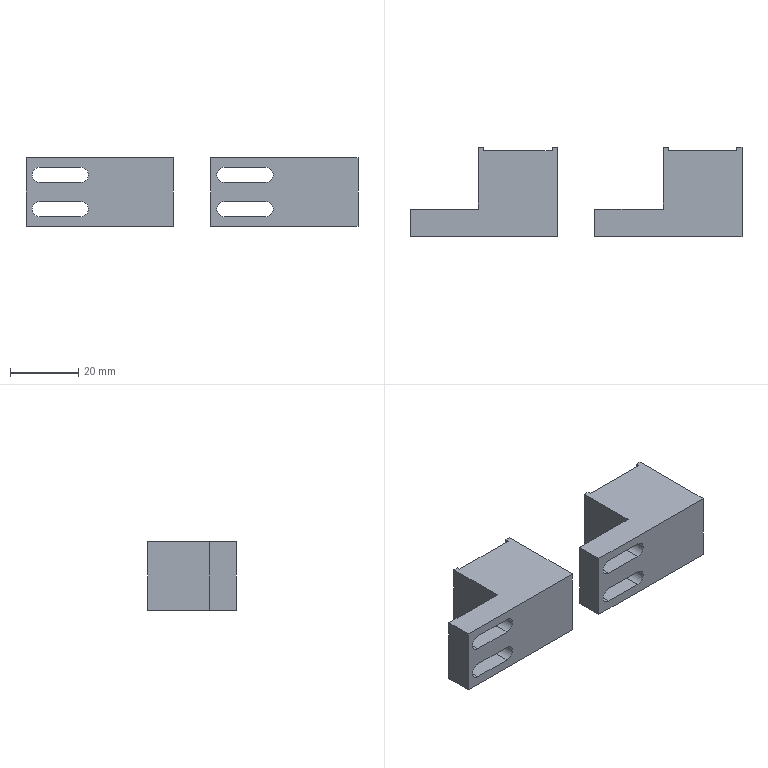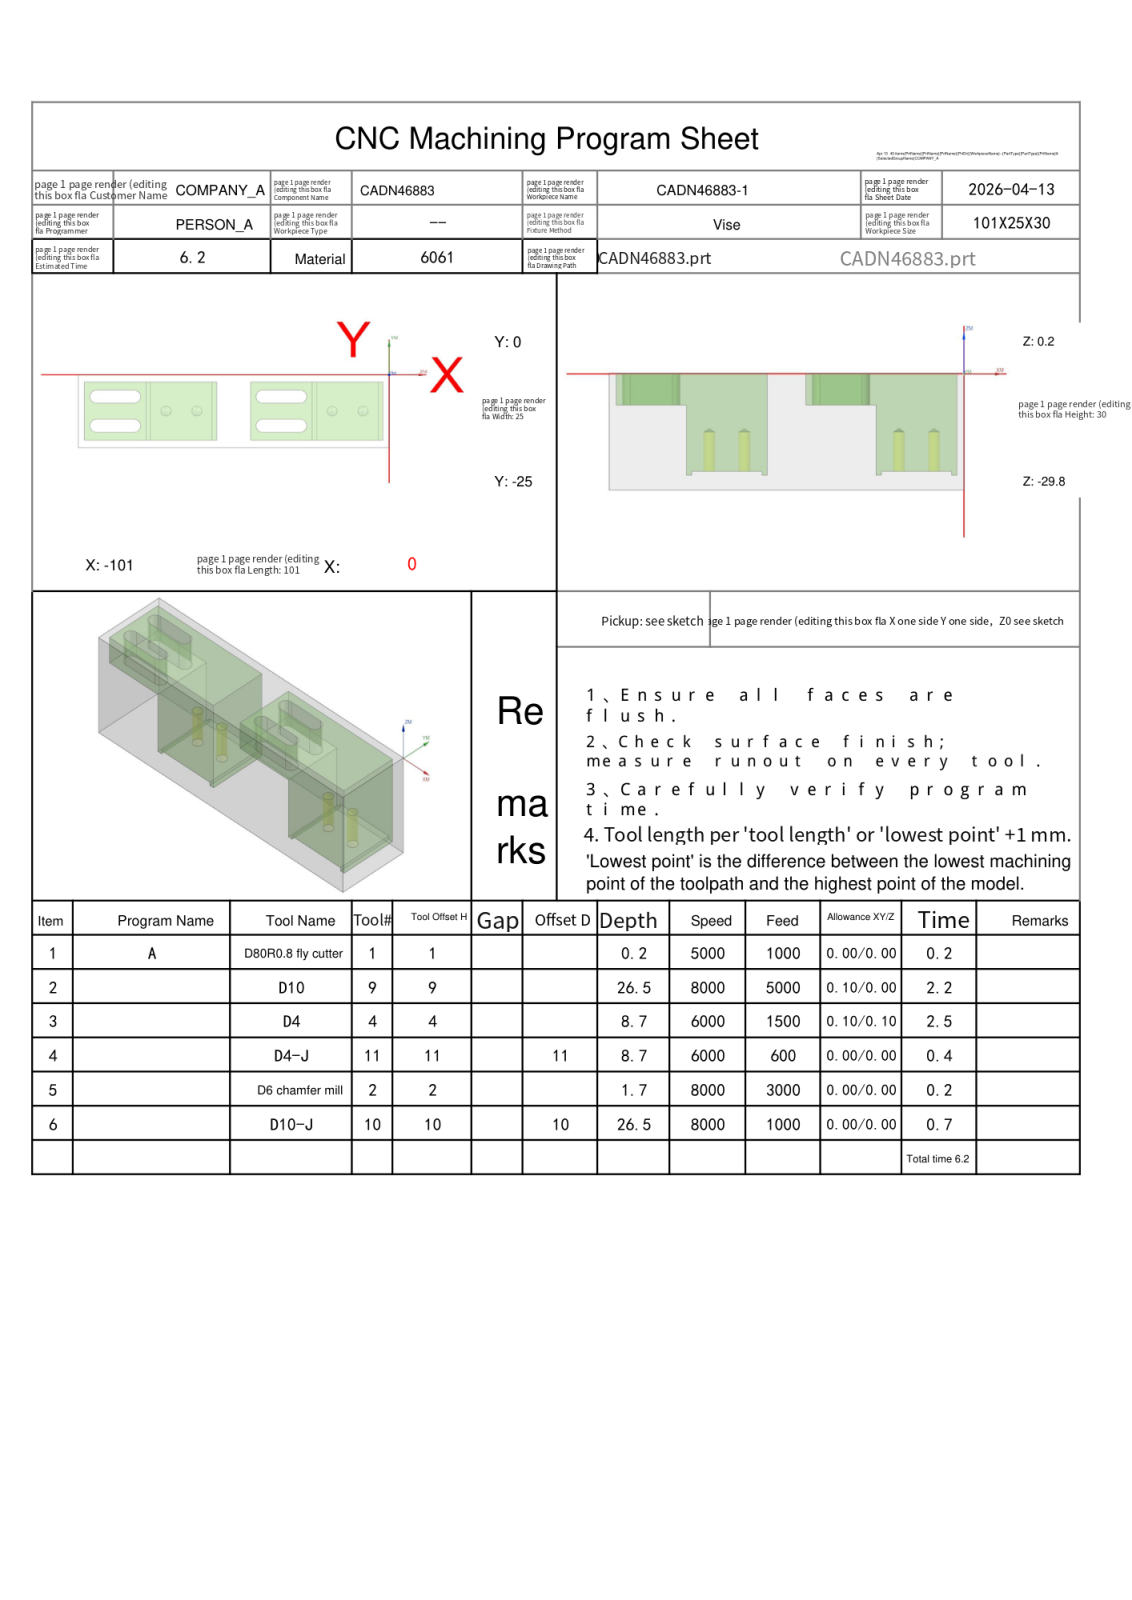NC program | NX | posted by the shop | part box 97 x 26 x 20 mm
Lines 1 to 1841 of 2082, first 1269 of 1839 lines:
%
O0001
(Machine time: 7.36 MIN)
(===Total Tool:6===)
(T1=D80R0.8 fly cutter D=80.  R=0.8  D-  H01 Z=0.    )
(T9=D10     D=10.  R=0.   D-  H09 Z=-26.3 )
(T4=D4      D=4.   R=0.   D-  H04 Z=-8.5  )
(T11=D4-J   D=4.   R=0.   D11 H11 Z=-8.5  )
(T2=D6 chamfer mill   D=6.   R=0.   D-  H02 Z=-1.5  )
(T10=D10-J  D=10.  R=0.   D10 H10 Z=-26.3 )
G80 G90 G17 G49 G40
G91 G28 Z0
M01
N1 T01 M06
(D80R0.8 fly cutter  D=80. R=0.8 H=01 ce=0.00 di=0.00)
(MAX_Z=20. MIN_Z=0. Time=0.20M)
G00 G90 G54 X43. Y-12.5 M03 S5000
G43 H01 Z20.
M08
Z2.
G01 Z0.0 F1000.
X38.
X-139.
X-144.
Z2.
G00 Z20.
G91 G28 Z0.0
M05
M09
G91 G28 Z0.0
M01
N2 T09 M06
(D10  D=10. R=0. H=09 ce=0.10 di=0.00)
(MAX_Z=20. MIN_Z=-26.3 Time=2.23M)
G00 G90 G54 X-77.5 Y-27.6 M03 S8000
G43 H09 Z20.
M08
Z.5
G01 X-99. Z.393 F5000.
G02 X-104.1 Y-22.5 Z.353 I0.0 J5.1
G01 Y-2.5 Z.253
G02 X-99. Y2.6 Z.213 I5.1 J0.0
G01 X-56. Z-.001
G02 X-50.9 Y-2.5 Z-.041 I0.0 J-5.1
G01 Y-22.5 Z-.141
G02 X-56. Y-27.6 Z-.181 I-5.1 J0.0
G01 X-99. Z-.395
G02 X-104.1 Y-22.5 Z-.435 I0.0 J5.1
G01 Y-2.5 Z-.535
G02 X-99. Y2.6 Z-.575 I5.1 J0.0
G01 X-56. Z-.79
G02 X-50.9 Y-2.5 Z-.83 I0.0 J-5.1
G01 Y-22.5 Z-.929
G02 X-56. Y-27.6 Z-.969 I-5.1 J0.0
G01 X-99. Z-1.184
G02 X-104.1 Y-22.5 Z-1.224 I0.0 J5.1
G01 Y-2.5 Z-1.323
G02 X-99. Y2.6 Z-1.363 I5.1 J0.0
G01 X-56. Z-1.578
G02 X-50.9 Y-2.5 Z-1.618 I0.0 J-5.1
G01 Y-22.5 Z-1.718
G02 X-56. Y-27.6 Z-1.757 I-5.1 J0.0
G01 X-99. Z-1.972
G02 X-104.1 Y-22.5 Z-2.012 I0.0 J5.1
G01 Y-2.5 Z-2.112
G02 X-99. Y2.6 Z-2.152 I5.1 J0.0
G01 X-56. Z-2.366
G02 X-50.9 Y-2.5 Z-2.406 I0.0 J-5.1
G01 Y-22.5 Z-2.506
G02 X-56. Y-27.6 Z-2.546 I-5.1 J0.0
G01 X-99. Z-2.76
G02 X-104.1 Y-22.5 Z-2.8 I0.0 J5.1
G01 Y-2.5 Z-2.9
G02 X-99. Y2.6 Z-2.94 I5.1 J0.0
G01 X-56. Z-3.154
G02 X-50.9 Y-2.5 Z-3.194 I0.0 J-5.1
G01 Y-22.5 Z-3.294
G02 X-56. Y-27.6 Z-3.334 I-5.1 J0.0
G01 X-99. Z-3.548
G02 X-104.1 Y-22.5 Z-3.588 I0.0 J5.1
G01 Y-2.5 Z-3.688
G02 X-99. Y2.6 Z-3.728 I5.1 J0.0
G01 X-56. Z-3.943
G02 X-50.9 Y-2.5 Z-3.982 I0.0 J-5.1
G01 Y-22.5 Z-4.082
G02 X-56. Y-27.6 Z-4.122 I-5.1 J0.0
G01 X-99. Z-4.337
G02 X-104.1 Y-22.5 Z-4.377 I0.0 J5.1
G01 Y-2.5 Z-4.476
G02 X-99. Y2.6 Z-4.516 I5.1 J0.0
G01 X-56. Z-4.731
G02 X-50.9 Y-2.5 Z-4.771 I0.0 J-5.1
G01 Y-22.5 Z-4.87
G02 X-56. Y-27.6 Z-4.91 I-5.1 J0.0
G01 X-99. Z-5.125
G02 X-104.1 Y-22.5 Z-5.165 I0.0 J5.1
G01 Y-2.5 Z-5.265
G02 X-99. Y2.6 Z-5.305 I5.1 J0.0
G01 X-56. Z-5.519
G02 X-50.9 Y-2.5 Z-5.559 I0.0 J-5.1
G01 Y-22.5 Z-5.659
G02 X-56. Y-27.6 Z-5.699 I-5.1 J0.0
G01 X-99. Z-5.913
G02 X-104.1 Y-22.5 Z-5.953 I0.0 J5.1
G01 Y-2.5 Z-6.053
G02 X-99. Y2.6 Z-6.093 I5.1 J0.0
G01 X-56. Z-6.307
G02 X-50.9 Y-2.5 Z-6.347 I0.0 J-5.1
G01 Y-22.5 Z-6.447
G02 X-56. Y-27.6 Z-6.487 I-5.1 J0.0
G01 X-99. Z-6.701
G02 X-104.1 Y-22.5 Z-6.741 I0.0 J5.1
G01 Y-2.5 Z-6.841
G02 X-99. Y2.6 Z-6.881 I5.1 J0.0
G01 X-56. Z-7.095
G02 X-50.9 Y-2.5 Z-7.135 I0.0 J-5.1
G01 Y-22.5 Z-7.235
G02 X-56. Y-27.6 Z-7.275 I-5.1 J0.0
G01 X-99. Z-7.49
G02 X-104.1 Y-22.5 Z-7.53 I0.0 J5.1
G01 Y-2.5 Z-7.629
G02 X-99. Y2.6 Z-7.669 I5.1 J0.0
G01 X-56. Z-7.884
G02 X-50.9 Y-2.5 Z-7.924 I0.0 J-5.1
G01 Y-22.5 Z-8.023
G02 X-56. Y-27.6 Z-8.063 I-5.1 J0.0
G01 X-99. Z-8.278
G02 X-104.1 Y-22.5 Z-8.318 I0.0 J5.1
G01 Y-2.5 Z-8.418
G02 X-99. Y2.6 Z-8.457 I5.1 J0.0
G01 X-56. Z-8.672
G02 X-50.9 Y-2.5 Z-8.712 I0.0 J-5.1
G01 Y-22.5 Z-8.812
G02 X-56. Y-27.6 Z-8.852 I-5.1 J0.0
G01 X-99. Z-9.066
G02 X-104.1 Y-22.5 Z-9.106 I0.0 J5.1
G01 Y-2.5 Z-9.206
G02 X-99. Y2.6 Z-9.246 I5.1 J0.0
G01 X-56. Z-9.46
G02 X-50.9 Y-2.5 Z-9.5 I0.0 J-5.1
G01 Y-22.5 Z-9.6
G02 X-56. Y-27.6 Z-9.64 I-5.1 J0.0
G01 X-99. Z-9.854
G02 X-104.1 Y-22.5 Z-9.894 I0.0 J5.1
G01 Y-2.5 Z-9.994
G02 X-99. Y2.6 Z-10.034 I5.1 J0.0
G01 X-56. Z-10.248
G02 X-50.9 Y-2.5 Z-10.288 I0.0 J-5.1
G01 Y-22.5 Z-10.388
G02 X-56. Y-27.6 Z-10.428 I-5.1 J0.0
G01 X-99. Z-10.643
G02 X-104.1 Y-22.5 Z-10.682 I0.0 J5.1
G01 Y-2.5 Z-10.782
G02 X-99. Y2.6 Z-10.822 I5.1 J0.0
G01 X-56. Z-11.037
G02 X-50.9 Y-2.5 Z-11.077 I0.0 J-5.1
G01 Y-22.5 Z-11.176
G02 X-56. Y-27.6 Z-11.216 I-5.1 J0.0
G01 X-99. Z-11.431
G02 X-104.1 Y-22.5 Z-11.471 I0.0 J5.1
G01 Y-2.5 Z-11.57
G02 X-99. Y2.6 Z-11.61 I5.1 J0.0
G01 X-56. Z-11.825
G02 X-50.9 Y-2.5 Z-11.865 I0.0 J-5.1
G01 Y-22.5 Z-11.965
G02 X-56. Y-27.6 Z-12.005 I-5.1 J0.0
G01 X-99. Z-12.219
G02 X-104.1 Y-22.5 Z-12.259 I0.0 J5.1
G01 Y-2.5 Z-12.359
G02 X-99. Y2.6 Z-12.399 I5.1 J0.0
G01 X-56. Z-12.613
G02 X-50.9 Y-2.5 Z-12.653 I0.0 J-5.1
G01 Y-22.5 Z-12.753
G02 X-56. Y-27.6 Z-12.793 I-5.1 J0.0
G01 X-99. Z-13.007
G02 X-104.1 Y-22.5 Z-13.047 I0.0 J5.1
G01 Y-2.5 Z-13.147
G02 X-99. Y2.6 Z-13.187 I5.1 J0.0
G01 X-56. Z-13.401
G02 X-50.9 Y-2.5 Z-13.441 I0.0 J-5.1
G01 Y-22.5 Z-13.541
G02 X-56. Y-27.6 Z-13.581 I-5.1 J0.0
G01 X-99. Z-13.795
G02 X-104.1 Y-22.5 Z-13.835 I0.0 J5.1
G01 Y-2.5 Z-13.935
G02 X-99. Y2.6 Z-13.975 I5.1 J0.0
G01 X-56. Z-14.19
G02 X-50.9 Y-2.5 Z-14.23 I0.0 J-5.1
G01 Y-22.5 Z-14.329
G02 X-56. Y-27.6 Z-14.369 I-5.1 J0.0
G01 X-99. Z-14.584
G02 X-104.1 Y-22.5 Z-14.624 I0.0 J5.1
G01 Y-2.5 Z-14.723
G02 X-99. Y2.6 Z-14.763 I5.1 J0.0
G01 X-56. Z-14.978
G02 X-50.9 Y-2.5 Z-15.018 I0.0 J-5.1
G01 Y-22.5 Z-15.118
G02 X-56. Y-27.6 Z-15.157 I-5.1 J0.0
G01 X-99. Z-15.372
G02 X-104.1 Y-22.5 Z-15.412 I0.0 J5.1
G01 Y-2.5 Z-15.512
G02 X-99. Y2.6 Z-15.552 I5.1 J0.0
G01 X-56. Z-15.766
G02 X-50.9 Y-2.5 Z-15.806 I0.0 J-5.1
G01 Y-22.5 Z-15.906
G02 X-56. Y-27.6 Z-15.946 I-5.1 J0.0
G01 X-99. Z-16.16
G02 X-104.1 Y-22.5 Z-16.2 I0.0 J5.1
G01 Y-2.5 Z-16.3
G02 X-99. Y2.6 Z-16.34 I5.1 J0.0
G01 X-56. Z-16.554
G02 X-50.9 Y-2.5 Z-16.594 I0.0 J-5.1
G01 Y-22.5 Z-16.694
G02 X-56. Y-27.6 Z-16.734 I-5.1 J0.0
G01 X-99. Z-16.948
G02 X-104.1 Y-22.5 Z-16.988 I0.0 J5.1
G01 Y-2.5 Z-17.088
G02 X-99. Y2.6 Z-17.128 I5.1 J0.0
G01 X-56. Z-17.343
G02 X-50.9 Y-2.5 Z-17.382 I0.0 J-5.1
G01 Y-22.5 Z-17.482
G02 X-56. Y-27.6 Z-17.522 I-5.1 J0.0
G01 X-99. Z-17.737
G02 X-104.1 Y-22.5 Z-17.777 I0.0 J5.1
G01 Y-2.5 Z-17.876
G02 X-99. Y2.6 Z-17.916 I5.1 J0.0
G01 X-56. Z-18.131
G02 X-50.9 Y-2.5 Z-18.171 I0.0 J-5.1
G01 Y-22.5 Z-18.27
G02 X-56. Y-27.6 Z-18.31 I-5.1 J0.0
G01 X-99. Z-18.525
G02 X-104.1 Y-22.5 Z-18.565 I0.0 J5.1
G01 Y-2.5 Z-18.665
G02 X-99. Y2.6 Z-18.705 I5.1 J0.0
G01 X-56. Z-18.919
G02 X-50.9 Y-2.5 Z-18.959 I0.0 J-5.1
G01 Y-22.5 Z-19.059
G02 X-56. Y-27.6 Z-19.099 I-5.1 J0.0
G01 X-99. Z-19.313
G02 X-104.1 Y-22.5 Z-19.353 I0.0 J5.1
G01 Y-2.5 Z-19.453
G02 X-99. Y2.6 Z-19.493 I5.1 J0.0
G01 X-56. Z-19.707
G02 X-50.9 Y-2.5 Z-19.747 I0.0 J-5.1
G01 Y-22.5 Z-19.847
G02 X-56. Y-27.6 Z-19.887 I-5.1 J0.0
G01 X-99. Z-20.101
G02 X-104.1 Y-22.5 Z-20.141 I0.0 J5.1
G01 Y-2.5 Z-20.241
G02 X-99. Y2.6 Z-20.281 I5.1 J0.0
G01 X-56. Z-20.495
G02 X-50.9 Y-2.5 Z-20.535 I0.0 J-5.1
G01 Y-22.5 Z-20.635
G02 X-56. Y-27.6 Z-20.675 I-5.1 J0.0
G01 X-99. Z-20.89
G02 X-104.1 Y-22.5 Z-20.93 I0.0 J5.1
G01 Y-2.5 Z-21.029
G02 X-99. Y2.6 Z-21.069 I5.1 J0.0
G01 X-56. Z-21.284
G02 X-50.9 Y-2.5 Z-21.324 I0.0 J-5.1
G01 Y-22.5 Z-21.423
G02 X-56. Y-27.6 Z-21.463 I-5.1 J0.0
G01 X-99. Z-21.678
G02 X-104.1 Y-22.5 Z-21.718 I0.0 J5.1
G01 Y-2.5 Z-21.818
G02 X-99. Y2.6 Z-21.857 I5.1 J0.0
G01 X-56. Z-22.072
G02 X-50.9 Y-2.5 Z-22.112 I0.0 J-5.1
G01 Y-22.5 Z-22.212
G02 X-56. Y-27.6 Z-22.252 I-5.1 J0.0
G01 X-99. Z-22.466
G02 X-104.1 Y-22.5 Z-22.506 I0.0 J5.1
G01 Y-2.5 Z-22.606
G02 X-99. Y2.6 Z-22.646 I5.1 J0.0
G01 X-56. Z-22.86
G02 X-50.9 Y-2.5 Z-22.9 I0.0 J-5.1
G01 Y-22.5 Z-23.
G02 X-56. Y-27.6 Z-23.04 I-5.1 J0.0
G01 X-99. Z-23.254
G02 X-104.1 Y-22.5 Z-23.294 I0.0 J5.1
G01 Y-2.5 Z-23.394
G02 X-99. Y2.6 Z-23.434 I5.1 J0.0
G01 X-56. Z-23.648
G02 X-50.9 Y-2.5 Z-23.688 I0.0 J-5.1
G01 Y-22.5 Z-23.788
G02 X-56. Y-27.6 Z-23.828 I-5.1 J0.0
G01 X-99. Z-24.043
G02 X-104.1 Y-22.5 Z-24.082 I0.0 J5.1
G01 Y-2.5 Z-24.182
G02 X-99. Y2.6 Z-24.222 I5.1 J0.0
G01 X-56. Z-24.437
G02 X-50.9 Y-2.5 Z-24.477 I0.0 J-5.1
G01 Y-22.5 Z-24.576
G02 X-56. Y-27.6 Z-24.616 I-5.1 J0.0
G01 X-99. Z-24.831
G02 X-104.1 Y-22.5 Z-24.871 I0.0 J5.1
G01 Y-2.5 Z-24.97
G02 X-99. Y2.6 Z-25.01 I5.1 J0.0
G01 X-56. Z-25.225
G02 X-50.9 Y-2.5 Z-25.265 I0.0 J-5.1
G01 Y-22.5 Z-25.365
G02 X-56. Y-27.6 Z-25.405 I-5.1 J0.0
G01 X-99. Z-25.619
G02 X-104.1 Y-22.5 Z-25.659 I0.0 J5.1
G01 Y-2.5 Z-25.759
G02 X-99. Y2.6 Z-25.799 I5.1 J0.0
G01 X-56. Z-26.013
G02 X-50.9 Y-2.5 Z-26.053 I0.0 J-5.1
G01 Y-22.5 Z-26.153
G02 X-56. Y-27.6 Z-26.193 I-5.1 J0.0
G01 X-77.5 Z-26.3
X-99.
G02 X-104.1 Y-22.5 I0.0 J5.1
G01 Y-2.5
G02 X-99. Y2.6 I5.1 J0.0
G01 X-56.
G02 X-50.9 Y-2.5 I0.0 J-5.1
G01 Y-22.5
G02 X-56. Y-27.6 I-5.1 J0.0
G01 X-77.5
X-78.
Z-25.3
G00 Z20.
X-23.5
Z.5
G01 X-45. Z.393
G02 X-50.1 Y-22.5 Z.353 I0.0 J5.1
G01 Y-2.5 Z.253
G02 X-45. Y2.6 Z.213 I5.1 J0.0
G01 X-2. Z-.001
G02 X3.1 Y-2.5 Z-.041 I0.0 J-5.1
G01 Y-22.5 Z-.141
G02 X-2. Y-27.6 Z-.181 I-5.1 J0.0
G01 X-45. Z-.395
G02 X-50.1 Y-22.5 Z-.435 I0.0 J5.1
G01 Y-2.5 Z-.535
G02 X-45. Y2.6 Z-.575 I5.1 J0.0
G01 X-2. Z-.79
G02 X3.1 Y-2.5 Z-.83 I0.0 J-5.1
G01 Y-22.5 Z-.929
G02 X-2. Y-27.6 Z-.969 I-5.1 J0.0
G01 X-45. Z-1.184
G02 X-50.1 Y-22.5 Z-1.224 I0.0 J5.1
G01 Y-2.5 Z-1.323
G02 X-45. Y2.6 Z-1.363 I5.1 J0.0
G01 X-2. Z-1.578
G02 X3.1 Y-2.5 Z-1.618 I0.0 J-5.1
G01 Y-22.5 Z-1.718
G02 X-2. Y-27.6 Z-1.757 I-5.1 J0.0
G01 X-45. Z-1.972
G02 X-50.1 Y-22.5 Z-2.012 I0.0 J5.1
G01 Y-2.5 Z-2.112
G02 X-45. Y2.6 Z-2.152 I5.1 J0.0
G01 X-2. Z-2.366
G02 X3.1 Y-2.5 Z-2.406 I0.0 J-5.1
G01 Y-22.5 Z-2.506
G02 X-2. Y-27.6 Z-2.546 I-5.1 J0.0
G01 X-45. Z-2.76
G02 X-50.1 Y-22.5 Z-2.8 I0.0 J5.1
G01 Y-2.5 Z-2.9
G02 X-45. Y2.6 Z-2.94 I5.1 J0.0
G01 X-2. Z-3.154
G02 X3.1 Y-2.5 Z-3.194 I0.0 J-5.1
G01 Y-22.5 Z-3.294
G02 X-2. Y-27.6 Z-3.334 I-5.1 J0.0
G01 X-45. Z-3.548
G02 X-50.1 Y-22.5 Z-3.588 I0.0 J5.1
G01 Y-2.5 Z-3.688
G02 X-45. Y2.6 Z-3.728 I5.1 J0.0
G01 X-2. Z-3.943
G02 X3.1 Y-2.5 Z-3.982 I0.0 J-5.1
G01 Y-22.5 Z-4.082
G02 X-2. Y-27.6 Z-4.122 I-5.1 J0.0
G01 X-45. Z-4.337
G02 X-50.1 Y-22.5 Z-4.377 I0.0 J5.1
G01 Y-2.5 Z-4.476
G02 X-45. Y2.6 Z-4.516 I5.1 J0.0
G01 X-2. Z-4.731
G02 X3.1 Y-2.5 Z-4.771 I0.0 J-5.1
G01 Y-22.5 Z-4.87
G02 X-2. Y-27.6 Z-4.91 I-5.1 J0.0
G01 X-45. Z-5.125
G02 X-50.1 Y-22.5 Z-5.165 I0.0 J5.1
G01 Y-2.5 Z-5.265
G02 X-45. Y2.6 Z-5.305 I5.1 J0.0
G01 X-2. Z-5.519
G02 X3.1 Y-2.5 Z-5.559 I0.0 J-5.1
G01 Y-22.5 Z-5.659
G02 X-2. Y-27.6 Z-5.699 I-5.1 J0.0
G01 X-45. Z-5.913
G02 X-50.1 Y-22.5 Z-5.953 I0.0 J5.1
G01 Y-2.5 Z-6.053
G02 X-45. Y2.6 Z-6.093 I5.1 J0.0
G01 X-2. Z-6.307
G02 X3.1 Y-2.5 Z-6.347 I0.0 J-5.1
G01 Y-22.5 Z-6.447
G02 X-2. Y-27.6 Z-6.487 I-5.1 J0.0
G01 X-45. Z-6.701
G02 X-50.1 Y-22.5 Z-6.741 I0.0 J5.1
G01 Y-2.5 Z-6.841
G02 X-45. Y2.6 Z-6.881 I5.1 J0.0
G01 X-2. Z-7.095
G02 X3.1 Y-2.5 Z-7.135 I0.0 J-5.1
G01 Y-22.5 Z-7.235
G02 X-2. Y-27.6 Z-7.275 I-5.1 J0.0
G01 X-45. Z-7.49
G02 X-50.1 Y-22.5 Z-7.53 I0.0 J5.1
G01 Y-2.5 Z-7.629
G02 X-45. Y2.6 Z-7.669 I5.1 J0.0
G01 X-2. Z-7.884
G02 X3.1 Y-2.5 Z-7.924 I0.0 J-5.1
G01 Y-22.5 Z-8.023
G02 X-2. Y-27.6 Z-8.063 I-5.1 J0.0
G01 X-45. Z-8.278
G02 X-50.1 Y-22.5 Z-8.318 I0.0 J5.1
G01 Y-2.5 Z-8.418
G02 X-45. Y2.6 Z-8.457 I5.1 J0.0
G01 X-2. Z-8.672
G02 X3.1 Y-2.5 Z-8.712 I0.0 J-5.1
G01 Y-22.5 Z-8.812
G02 X-2. Y-27.6 Z-8.852 I-5.1 J0.0
G01 X-45. Z-9.066
G02 X-50.1 Y-22.5 Z-9.106 I0.0 J5.1
G01 Y-2.5 Z-9.206
G02 X-45. Y2.6 Z-9.246 I5.1 J0.0
G01 X-2. Z-9.46
G02 X3.1 Y-2.5 Z-9.5 I0.0 J-5.1
G01 Y-22.5 Z-9.6
G02 X-2. Y-27.6 Z-9.64 I-5.1 J0.0
G01 X-45. Z-9.854
G02 X-50.1 Y-22.5 Z-9.894 I0.0 J5.1
G01 Y-2.5 Z-9.994
G02 X-45. Y2.6 Z-10.034 I5.1 J0.0
G01 X-2. Z-10.248
G02 X3.1 Y-2.5 Z-10.288 I0.0 J-5.1
G01 Y-22.5 Z-10.388
G02 X-2. Y-27.6 Z-10.428 I-5.1 J0.0
G01 X-45. Z-10.643
G02 X-50.1 Y-22.5 Z-10.682 I0.0 J5.1
G01 Y-2.5 Z-10.782
G02 X-45. Y2.6 Z-10.822 I5.1 J0.0
G01 X-2. Z-11.037
G02 X3.1 Y-2.5 Z-11.077 I0.0 J-5.1
G01 Y-22.5 Z-11.176
G02 X-2. Y-27.6 Z-11.216 I-5.1 J0.0
G01 X-45. Z-11.431
G02 X-50.1 Y-22.5 Z-11.471 I0.0 J5.1
G01 Y-2.5 Z-11.57
G02 X-45. Y2.6 Z-11.61 I5.1 J0.0
G01 X-2. Z-11.825
G02 X3.1 Y-2.5 Z-11.865 I0.0 J-5.1
G01 Y-22.5 Z-11.965
G02 X-2. Y-27.6 Z-12.005 I-5.1 J0.0
G01 X-45. Z-12.219
G02 X-50.1 Y-22.5 Z-12.259 I0.0 J5.1
G01 Y-2.5 Z-12.359
G02 X-45. Y2.6 Z-12.399 I5.1 J0.0
G01 X-2. Z-12.613
G02 X3.1 Y-2.5 Z-12.653 I0.0 J-5.1
G01 Y-22.5 Z-12.753
G02 X-2. Y-27.6 Z-12.793 I-5.1 J0.0
G01 X-45. Z-13.007
G02 X-50.1 Y-22.5 Z-13.047 I0.0 J5.1
G01 Y-2.5 Z-13.147
G02 X-45. Y2.6 Z-13.187 I5.1 J0.0
G01 X-2. Z-13.401
G02 X3.1 Y-2.5 Z-13.441 I0.0 J-5.1
G01 Y-22.5 Z-13.541
G02 X-2. Y-27.6 Z-13.581 I-5.1 J0.0
G01 X-45. Z-13.795
G02 X-50.1 Y-22.5 Z-13.835 I0.0 J5.1
G01 Y-2.5 Z-13.935
G02 X-45. Y2.6 Z-13.975 I5.1 J0.0
G01 X-2. Z-14.19
G02 X3.1 Y-2.5 Z-14.23 I0.0 J-5.1
G01 Y-22.5 Z-14.329
G02 X-2. Y-27.6 Z-14.369 I-5.1 J0.0
G01 X-45. Z-14.584
G02 X-50.1 Y-22.5 Z-14.624 I0.0 J5.1
G01 Y-2.5 Z-14.723
G02 X-45. Y2.6 Z-14.763 I5.1 J0.0
G01 X-2. Z-14.978
G02 X3.1 Y-2.5 Z-15.018 I0.0 J-5.1
G01 Y-22.5 Z-15.118
G02 X-2. Y-27.6 Z-15.157 I-5.1 J0.0
G01 X-45. Z-15.372
G02 X-50.1 Y-22.5 Z-15.412 I0.0 J5.1
G01 Y-2.5 Z-15.512
G02 X-45. Y2.6 Z-15.552 I5.1 J0.0
G01 X-2. Z-15.766
G02 X3.1 Y-2.5 Z-15.806 I0.0 J-5.1
G01 Y-22.5 Z-15.906
G02 X-2. Y-27.6 Z-15.946 I-5.1 J0.0
G01 X-45. Z-16.16
G02 X-50.1 Y-22.5 Z-16.2 I0.0 J5.1
G01 Y-2.5 Z-16.3
G02 X-45. Y2.6 Z-16.34 I5.1 J0.0
G01 X-2. Z-16.554
G02 X3.1 Y-2.5 Z-16.594 I0.0 J-5.1
G01 Y-22.5 Z-16.694
G02 X-2. Y-27.6 Z-16.734 I-5.1 J0.0
G01 X-45. Z-16.948
G02 X-50.1 Y-22.5 Z-16.988 I0.0 J5.1
G01 Y-2.5 Z-17.088
G02 X-45. Y2.6 Z-17.128 I5.1 J0.0
G01 X-2. Z-17.343
G02 X3.1 Y-2.5 Z-17.382 I0.0 J-5.1
G01 Y-22.5 Z-17.482
G02 X-2. Y-27.6 Z-17.522 I-5.1 J0.0
G01 X-45. Z-17.737
G02 X-50.1 Y-22.5 Z-17.777 I0.0 J5.1
G01 Y-2.5 Z-17.876
G02 X-45. Y2.6 Z-17.916 I5.1 J0.0
G01 X-2. Z-18.131
G02 X3.1 Y-2.5 Z-18.171 I0.0 J-5.1
G01 Y-22.5 Z-18.27
G02 X-2. Y-27.6 Z-18.31 I-5.1 J0.0
G01 X-45. Z-18.525
G02 X-50.1 Y-22.5 Z-18.565 I0.0 J5.1
G01 Y-2.5 Z-18.665
G02 X-45. Y2.6 Z-18.705 I5.1 J0.0
G01 X-2. Z-18.919
G02 X3.1 Y-2.5 Z-18.959 I0.0 J-5.1
G01 Y-22.5 Z-19.059
G02 X-2. Y-27.6 Z-19.099 I-5.1 J0.0
G01 X-45. Z-19.313
G02 X-50.1 Y-22.5 Z-19.353 I0.0 J5.1
G01 Y-2.5 Z-19.453
G02 X-45. Y2.6 Z-19.493 I5.1 J0.0
G01 X-2. Z-19.707
G02 X3.1 Y-2.5 Z-19.747 I0.0 J-5.1
G01 Y-22.5 Z-19.847
G02 X-2. Y-27.6 Z-19.887 I-5.1 J0.0
G01 X-45. Z-20.101
G02 X-50.1 Y-22.5 Z-20.141 I0.0 J5.1
G01 Y-2.5 Z-20.241
G02 X-45. Y2.6 Z-20.281 I5.1 J0.0
G01 X-2. Z-20.495
G02 X3.1 Y-2.5 Z-20.535 I0.0 J-5.1
G01 Y-22.5 Z-20.635
G02 X-2. Y-27.6 Z-20.675 I-5.1 J0.0
G01 X-45. Z-20.89
G02 X-50.1 Y-22.5 Z-20.93 I0.0 J5.1
G01 Y-2.5 Z-21.029
G02 X-45. Y2.6 Z-21.069 I5.1 J0.0
G01 X-2. Z-21.284
G02 X3.1 Y-2.5 Z-21.324 I0.0 J-5.1
G01 Y-22.5 Z-21.423
G02 X-2. Y-27.6 Z-21.463 I-5.1 J0.0
G01 X-45. Z-21.678
G02 X-50.1 Y-22.5 Z-21.718 I0.0 J5.1
G01 Y-2.5 Z-21.818
G02 X-45. Y2.6 Z-21.857 I5.1 J0.0
G01 X-2. Z-22.072
G02 X3.1 Y-2.5 Z-22.112 I0.0 J-5.1
G01 Y-22.5 Z-22.212
G02 X-2. Y-27.6 Z-22.252 I-5.1 J0.0
G01 X-45. Z-22.466
G02 X-50.1 Y-22.5 Z-22.506 I0.0 J5.1
G01 Y-2.5 Z-22.606
G02 X-45. Y2.6 Z-22.646 I5.1 J0.0
G01 X-2. Z-22.86
G02 X3.1 Y-2.5 Z-22.9 I0.0 J-5.1
G01 Y-22.5 Z-23.
G02 X-2. Y-27.6 Z-23.04 I-5.1 J0.0
G01 X-45. Z-23.254
G02 X-50.1 Y-22.5 Z-23.294 I0.0 J5.1
G01 Y-2.5 Z-23.394
G02 X-45. Y2.6 Z-23.434 I5.1 J0.0
G01 X-2. Z-23.648
G02 X3.1 Y-2.5 Z-23.688 I0.0 J-5.1
G01 Y-22.5 Z-23.788
G02 X-2. Y-27.6 Z-23.828 I-5.1 J0.0
G01 X-45. Z-24.043
G02 X-50.1 Y-22.5 Z-24.082 I0.0 J5.1
G01 Y-2.5 Z-24.182
G02 X-45. Y2.6 Z-24.222 I5.1 J0.0
G01 X-2. Z-24.437
G02 X3.1 Y-2.5 Z-24.477 I0.0 J-5.1
G01 Y-22.5 Z-24.576
G02 X-2. Y-27.6 Z-24.616 I-5.1 J0.0
G01 X-45. Z-24.831
G02 X-50.1 Y-22.5 Z-24.871 I0.0 J5.1
G01 Y-2.5 Z-24.97
G02 X-45. Y2.6 Z-25.01 I5.1 J0.0
G01 X-2. Z-25.225
G02 X3.1 Y-2.5 Z-25.265 I0.0 J-5.1
G01 Y-22.5 Z-25.365
G02 X-2. Y-27.6 Z-25.405 I-5.1 J0.0
G01 X-45. Z-25.619
G02 X-50.1 Y-22.5 Z-25.659 I0.0 J5.1
G01 Y-2.5 Z-25.759
G02 X-45. Y2.6 Z-25.799 I5.1 J0.0
G01 X-2. Z-26.013
G02 X3.1 Y-2.5 Z-26.053 I0.0 J-5.1
G01 Y-22.5 Z-26.153
G02 X-2. Y-27.6 Z-26.193 I-5.1 J0.0
G01 X-23.5 Z-26.3
X-45.
G02 X-50.1 Y-22.5 I0.0 J5.1
G01 Y-2.5
G02 X-45. Y2.6 I5.1 J0.0
G01 X-2.
G02 X3.1 Y-2.5 I0.0 J-5.1
G01 Y-22.5
G02 X-2. Y-27.6 I-5.1 J0.0
G01 X-23.5
X-24.
Z-25.3
G00 Z20.
G91 G28 Z0.0
M05
M09
G91 G28 Z0.0
M01
N3 T04 M06
(D4  D=4. R=0. H=04 ce=0.10 di=0.10)
(MAX_Z=20. MIN_Z=-8.5 Time=2.49M)
G00 G90 G54 X-89. Y-17.65 M03 S6000
G43 H04 Z20.
M08
Z.5
G01 X-83. Z.44 F1500.
G03 X-82.85 Y-17.5 Z.438 I0.0 J.15
X-83. Y-17.35 Z.435 I-.15 J0.0
G01 X-95. Z.315
G03 X-95.15 Y-17.5 Z.313 I0.0 J-.15
X-95. Y-17.65 Z.31 I.15 J0.0
G01 X-83. Z.19
G03 X-82.85 Y-17.5 Z.188 I0.0 J.15
X-83. Y-17.35 Z.185 I-.15 J0.0
G01 X-95. Z.065
G03 X-95.15 Y-17.5 Z.063 I0.0 J-.15
X-95. Y-17.65 Z.06 I.15 J0.0
G01 X-83. Z-.06
G03 X-82.85 Y-17.5 Z-.063 I0.0 J.15
X-83. Y-17.35 Z-.065 I-.15 J0.0
G01 X-95. Z-.185
G03 X-95.15 Y-17.5 Z-.188 I0.0 J-.15
X-95. Y-17.65 Z-.19 I.15 J0.0
G01 X-83. Z-.31
G03 X-82.85 Y-17.5 Z-.313 I0.0 J.15
X-83. Y-17.35 Z-.315 I-.15 J0.0
G01 X-95. Z-.435
G03 X-95.15 Y-17.5 Z-.438 I0.0 J-.15
X-95. Y-17.65 Z-.44 I.15 J0.0
G01 X-83. Z-.56
G03 X-82.85 Y-17.5 Z-.563 I0.0 J.15
X-83. Y-17.35 Z-.565 I-.15 J0.0
G01 X-95. Z-.685
G03 X-95.15 Y-17.5 Z-.688 I0.0 J-.15
X-95. Y-17.65 Z-.69 I.15 J0.0
G01 X-83. Z-.81
G03 X-82.85 Y-17.5 Z-.813 I0.0 J.15
X-83. Y-17.35 Z-.815 I-.15 J0.0
G01 X-95. Z-.935
G03 X-95.15 Y-17.5 Z-.938 I0.0 J-.15
X-95. Y-17.65 Z-.94 I.15 J0.0
G01 X-83. Z-1.06
G03 X-82.85 Y-17.5 Z-1.063 I0.0 J.15
X-83. Y-17.35 Z-1.065 I-.15 J0.0
G01 X-95. Z-1.185
G03 X-95.15 Y-17.5 Z-1.188 I0.0 J-.15
X-95. Y-17.65 Z-1.19 I.15 J0.0
G01 X-83. Z-1.31
G03 X-82.85 Y-17.5 Z-1.313 I0.0 J.15
X-83. Y-17.35 Z-1.315 I-.15 J0.0
G01 X-95. Z-1.435
G03 X-95.15 Y-17.5 Z-1.438 I0.0 J-.15
X-95. Y-17.65 Z-1.44 I.15 J0.0
G01 X-83. Z-1.56
G03 X-82.85 Y-17.5 Z-1.563 I0.0 J.15
X-83. Y-17.35 Z-1.565 I-.15 J0.0
G01 X-95. Z-1.685
G03 X-95.15 Y-17.5 Z-1.688 I0.0 J-.15
X-95. Y-17.65 Z-1.69 I.15 J0.0
G01 X-83. Z-1.81
G03 X-82.85 Y-17.5 Z-1.813 I0.0 J.15
X-83. Y-17.35 Z-1.815 I-.15 J0.0
G01 X-95. Z-1.935
G03 X-95.15 Y-17.5 Z-1.938 I0.0 J-.15
X-95. Y-17.65 Z-1.94 I.15 J0.0
G01 X-83. Z-2.06
G03 X-82.85 Y-17.5 Z-2.063 I0.0 J.15
X-83. Y-17.35 Z-2.065 I-.15 J0.0
G01 X-95. Z-2.185
G03 X-95.15 Y-17.5 Z-2.188 I0.0 J-.15
X-95. Y-17.65 Z-2.19 I.15 J0.0
G01 X-83. Z-2.31
G03 X-82.85 Y-17.5 Z-2.313 I0.0 J.15
X-83. Y-17.35 Z-2.315 I-.15 J0.0
G01 X-95. Z-2.435
G03 X-95.15 Y-17.5 Z-2.438 I0.0 J-.15
X-95. Y-17.65 Z-2.44 I.15 J0.0
G01 X-83. Z-2.56
G03 X-82.85 Y-17.5 Z-2.563 I0.0 J.15
X-83. Y-17.35 Z-2.565 I-.15 J0.0
G01 X-95. Z-2.685
G03 X-95.15 Y-17.5 Z-2.688 I0.0 J-.15
X-95. Y-17.65 Z-2.69 I.15 J0.0
G01 X-83. Z-2.81
G03 X-82.85 Y-17.5 Z-2.813 I0.0 J.15
X-83. Y-17.35 Z-2.815 I-.15 J0.0
G01 X-95. Z-2.935
G03 X-95.15 Y-17.5 Z-2.938 I0.0 J-.15
X-95. Y-17.65 Z-2.94 I.15 J0.0
G01 X-83. Z-3.06
G03 X-82.85 Y-17.5 Z-3.063 I0.0 J.15
X-83. Y-17.35 Z-3.065 I-.15 J0.0
G01 X-95. Z-3.185
G03 X-95.15 Y-17.5 Z-3.188 I0.0 J-.15
X-95. Y-17.65 Z-3.19 I.15 J0.0
G01 X-83. Z-3.31
G03 X-82.85 Y-17.5 Z-3.313 I0.0 J.15
X-83. Y-17.35 Z-3.315 I-.15 J0.0
G01 X-95. Z-3.435
G03 X-95.15 Y-17.5 Z-3.438 I0.0 J-.15
X-95. Y-17.65 Z-3.44 I.15 J0.0
G01 X-83. Z-3.56
G03 X-82.85 Y-17.5 Z-3.563 I0.0 J.15
X-83. Y-17.35 Z-3.565 I-.15 J0.0
G01 X-95. Z-3.685
G03 X-95.15 Y-17.5 Z-3.688 I0.0 J-.15
X-95. Y-17.65 Z-3.69 I.15 J0.0
G01 X-83. Z-3.81
G03 X-82.85 Y-17.5 Z-3.813 I0.0 J.15
X-83. Y-17.35 Z-3.815 I-.15 J0.0
G01 X-95. Z-3.935
G03 X-95.15 Y-17.5 Z-3.938 I0.0 J-.15
X-95. Y-17.65 Z-3.94 I.15 J0.0
G01 X-83. Z-4.06
G03 X-82.85 Y-17.5 Z-4.063 I0.0 J.15
X-83. Y-17.35 Z-4.065 I-.15 J0.0
G01 X-95. Z-4.185
G03 X-95.15 Y-17.5 Z-4.188 I0.0 J-.15
X-95. Y-17.65 Z-4.19 I.15 J0.0
G01 X-83. Z-4.31
G03 X-82.85 Y-17.5 Z-4.313 I0.0 J.15
X-83. Y-17.35 Z-4.315 I-.15 J0.0
G01 X-95. Z-4.435
G03 X-95.15 Y-17.5 Z-4.438 I0.0 J-.15
X-95. Y-17.65 Z-4.44 I.15 J0.0
G01 X-83. Z-4.56
G03 X-82.85 Y-17.5 Z-4.563 I0.0 J.15
X-83. Y-17.35 Z-4.565 I-.15 J0.0
G01 X-95. Z-4.685
G03 X-95.15 Y-17.5 Z-4.688 I0.0 J-.15
X-95. Y-17.65 Z-4.69 I.15 J0.0
G01 X-83. Z-4.81
G03 X-82.85 Y-17.5 Z-4.813 I0.0 J.15
X-83. Y-17.35 Z-4.815 I-.15 J0.0
G01 X-95. Z-4.935
G03 X-95.15 Y-17.5 Z-4.938 I0.0 J-.15
X-95. Y-17.65 Z-4.94 I.15 J0.0
G01 X-83. Z-5.06
G03 X-82.85 Y-17.5 Z-5.063 I0.0 J.15
X-83. Y-17.35 Z-5.065 I-.15 J0.0
G01 X-95. Z-5.185
G03 X-95.15 Y-17.5 Z-5.188 I0.0 J-.15
X-95. Y-17.65 Z-5.19 I.15 J0.0
G01 X-83. Z-5.31
G03 X-82.85 Y-17.5 Z-5.313 I0.0 J.15
X-83. Y-17.35 Z-5.315 I-.15 J0.0
G01 X-95. Z-5.435
G03 X-95.15 Y-17.5 Z-5.438 I0.0 J-.15
X-95. Y-17.65 Z-5.44 I.15 J0.0
G01 X-83. Z-5.56
G03 X-82.85 Y-17.5 Z-5.563 I0.0 J.15
X-83. Y-17.35 Z-5.565 I-.15 J0.0
G01 X-95. Z-5.685
G03 X-95.15 Y-17.5 Z-5.688 I0.0 J-.15
X-95. Y-17.65 Z-5.69 I.15 J0.0
G01 X-83. Z-5.81
G03 X-82.85 Y-17.5 Z-5.813 I0.0 J.15
X-83. Y-17.35 Z-5.815 I-.15 J0.0
G01 X-95. Z-5.935
G03 X-95.15 Y-17.5 Z-5.938 I0.0 J-.15
X-95. Y-17.65 Z-5.94 I.15 J0.0
G01 X-83. Z-6.06
G03 X-82.85 Y-17.5 Z-6.063 I0.0 J.15
X-83. Y-17.35 Z-6.065 I-.15 J0.0
G01 X-95. Z-6.185
G03 X-95.15 Y-17.5 Z-6.188 I0.0 J-.15
X-95. Y-17.65 Z-6.19 I.15 J0.0
G01 X-83. Z-6.31
G03 X-82.85 Y-17.5 Z-6.313 I0.0 J.15
X-83. Y-17.35 Z-6.315 I-.15 J0.0
G01 X-95. Z-6.435
G03 X-95.15 Y-17.5 Z-6.438 I0.0 J-.15
X-95. Y-17.65 Z-6.44 I.15 J0.0
G01 X-83. Z-6.56
G03 X-82.85 Y-17.5 Z-6.563 I0.0 J.15
X-83. Y-17.35 Z-6.565 I-.15 J0.0
G01 X-95. Z-6.685
G03 X-95.15 Y-17.5 Z-6.688 I0.0 J-.15
X-95. Y-17.65 Z-6.69 I.15 J0.0
G01 X-83. Z-6.81
G03 X-82.85 Y-17.5 Z-6.813 I0.0 J.15
X-83. Y-17.35 Z-6.815 I-.15 J0.0
G01 X-95. Z-6.935
G03 X-95.15 Y-17.5 Z-6.938 I0.0 J-.15
X-95. Y-17.65 Z-6.94 I.15 J0.0
G01 X-83. Z-7.06
G03 X-82.85 Y-17.5 Z-7.063 I0.0 J.15
X-83. Y-17.35 Z-7.065 I-.15 J0.0
G01 X-95. Z-7.185
G03 X-95.15 Y-17.5 Z-7.188 I0.0 J-.15
X-95. Y-17.65 Z-7.19 I.15 J0.0
G01 X-83. Z-7.31
G03 X-82.85 Y-17.5 Z-7.313 I0.0 J.15
X-83. Y-17.35 Z-7.315 I-.15 J0.0
G01 X-95. Z-7.435
G03 X-95.15 Y-17.5 Z-7.438 I0.0 J-.15
X-95. Y-17.65 Z-7.44 I.15 J0.0
G01 X-83. Z-7.56
G03 X-82.85 Y-17.5 Z-7.563 I0.0 J.15
X-83. Y-17.35 Z-7.565 I-.15 J0.0
G01 X-95. Z-7.685
G03 X-95.15 Y-17.5 Z-7.688 I0.0 J-.15
X-95. Y-17.65 Z-7.69 I.15 J0.0
G01 X-83. Z-7.81
G03 X-82.85 Y-17.5 Z-7.813 I0.0 J.15
X-83. Y-17.35 Z-7.815 I-.15 J0.0
G01 X-95. Z-7.935
G03 X-95.15 Y-17.5 Z-7.938 I0.0 J-.15
X-95. Y-17.65 Z-7.94 I.15 J0.0
G01 X-83. Z-8.06
G03 X-82.85 Y-17.5 Z-8.063 I0.0 J.15
X-83. Y-17.35 Z-8.065 I-.15 J0.0
G01 X-95. Z-8.185
G03 X-95.15 Y-17.5 Z-8.188 I0.0 J-.15
X-95. Y-17.65 Z-8.19 I.15 J0.0
G01 X-83. Z-8.31
G03 X-82.85 Y-17.5 Z-8.313 I0.0 J.15
X-83. Y-17.35 Z-8.315 I-.15 J0.0
G01 X-95. Z-8.435
G03 X-95.15 Y-17.5 Z-8.438 I0.0 J-.15
X-95. Y-17.65 Z-8.44 I.15 J0.0
G01 X-89. Z-8.5
X-83.
G03 X-82.85 Y-17.5 I0.0 J.15
X-83. Y-17.35 I-.15 J0.0
G01 X-95.
G03 X-95.15 Y-17.5 I0.0 J-.15
X-95. Y-17.65 I.15 J0.0
G01 X-89.
X-88.5
Z-7.5
G00 Z20.
X-89. Y-7.35
Z.5
G01 X-95. Z.44
G03 X-95.15 Y-7.5 Z.438 I0.0 J-.15
X-95. Y-7.65 Z.435 I.15 J0.0
G01 X-83. Z.315
G03 X-82.85 Y-7.5 Z.313 I0.0 J.15
X-83. Y-7.35 Z.31 I-.15 J0.0
G01 X-95. Z.19
G03 X-95.15 Y-7.5 Z.188 I0.0 J-.15
X-95. Y-7.65 Z.185 I.15 J0.0
G01 X-83. Z.065
G03 X-82.85 Y-7.5 Z.063 I0.0 J.15
X-83. Y-7.35 Z.06 I-.15 J0.0
G01 X-95. Z-.06
G03 X-95.15 Y-7.5 Z-.063 I0.0 J-.15
X-95. Y-7.65 Z-.065 I.15 J0.0
G01 X-83. Z-.185
G03 X-82.85 Y-7.5 Z-.188 I0.0 J.15
X-83. Y-7.35 Z-.19 I-.15 J0.0
G01 X-95. Z-.31
G03 X-95.15 Y-7.5 Z-.313 I0.0 J-.15
X-95. Y-7.65 Z-.315 I.15 J0.0
G01 X-83. Z-.435
G03 X-82.85 Y-7.5 Z-.438 I0.0 J.15
X-83. Y-7.35 Z-.44 I-.15 J0.0
G01 X-95. Z-.56
G03 X-95.15 Y-7.5 Z-.563 I0.0 J-.15
X-95. Y-7.65 Z-.565 I.15 J0.0
G01 X-83. Z-.685
G03 X-82.85 Y-7.5 Z-.688 I0.0 J.15
X-83. Y-7.35 Z-.69 I-.15 J0.0
G01 X-95. Z-.81
G03 X-95.15 Y-7.5 Z-.813 I0.0 J-.15
X-95. Y-7.65 Z-.815 I.15 J0.0
G01 X-83. Z-.935
G03 X-82.85 Y-7.5 Z-.938 I0.0 J.15
X-83. Y-7.35 Z-.94 I-.15 J0.0
G01 X-95. Z-1.06
G03 X-95.15 Y-7.5 Z-1.063 I0.0 J-.15
X-95. Y-7.65 Z-1.065 I.15 J0.0
G01 X-83. Z-1.185
G03 X-82.85 Y-7.5 Z-1.188 I0.0 J.15
X-83. Y-7.35 Z-1.19 I-.15 J0.0
G01 X-95. Z-1.31
G03 X-95.15 Y-7.5 Z-1.313 I0.0 J-.15
X-95. Y-7.65 Z-1.315 I.15 J0.0
G01 X-83. Z-1.435
G03 X-82.85 Y-7.5 Z-1.438 I0.0 J.15
X-83. Y-7.35 Z-1.44 I-.15 J0.0
G01 X-95. Z-1.56
G03 X-95.15 Y-7.5 Z-1.563 I0.0 J-.15
X-95. Y-7.65 Z-1.565 I.15 J0.0
G01 X-83. Z-1.685
G03 X-82.85 Y-7.5 Z-1.688 I0.0 J.15
X-83. Y-7.35 Z-1.69 I-.15 J0.0
G01 X-95. Z-1.81
G03 X-95.15 Y-7.5 Z-1.813 I0.0 J-.15
X-95. Y-7.65 Z-1.815 I.15 J0.0
G01 X-83. Z-1.935
G03 X-82.85 Y-7.5 Z-1.938 I0.0 J.15
X-83. Y-7.35 Z-1.94 I-.15 J0.0
G01 X-95. Z-2.06
G03 X-95.15 Y-7.5 Z-2.063 I0.0 J-.15
X-95. Y-7.65 Z-2.065 I.15 J0.0
G01 X-83. Z-2.185
G03 X-82.85 Y-7.5 Z-2.188 I0.0 J.15
X-83. Y-7.35 Z-2.19 I-.15 J0.0
G01 X-95. Z-2.31
G03 X-95.15 Y-7.5 Z-2.313 I0.0 J-.15
X-95. Y-7.65 Z-2.315 I.15 J0.0
G01 X-83. Z-2.435
G03 X-82.85 Y-7.5 Z-2.438 I0.0 J.15
X-83. Y-7.35 Z-2.44 I-.15 J0.0
G01 X-95. Z-2.56
G03 X-95.15 Y-7.5 Z-2.563 I0.0 J-.15
X-95. Y-7.65 Z-2.565 I.15 J0.0
G01 X-83. Z-2.685
G03 X-82.85 Y-7.5 Z-2.688 I0.0 J.15
X-83. Y-7.35 Z-2.69 I-.15 J0.0
G01 X-95. Z-2.81
G03 X-95.15 Y-7.5 Z-2.813 I0.0 J-.15
X-95. Y-7.65 Z-2.815 I.15 J0.0
G01 X-83. Z-2.935
G03 X-82.85 Y-7.5 Z-2.938 I0.0 J.15
X-83. Y-7.35 Z-2.94 I-.15 J0.0
G01 X-95. Z-3.06
G03 X-95.15 Y-7.5 Z-3.063 I0.0 J-.15
X-95. Y-7.65 Z-3.065 I.15 J0.0
G01 X-83. Z-3.185
G03 X-82.85 Y-7.5 Z-3.188 I0.0 J.15
X-83. Y-7.35 Z-3.19 I-.15 J0.0
G01 X-95. Z-3.31
G03 X-95.15 Y-7.5 Z-3.313 I0.0 J-.15
X-95. Y-7.65 Z-3.315 I.15 J0.0
G01 X-83. Z-3.435
G03 X-82.85 Y-7.5 Z-3.438 I0.0 J.15
X-83. Y-7.35 Z-3.44 I-.15 J0.0
G01 X-95. Z-3.56
G03 X-95.15 Y-7.5 Z-3.563 I0.0 J-.15
X-95. Y-7.65 Z-3.565 I.15 J0.0
G01 X-83. Z-3.685
G03 X-82.85 Y-7.5 Z-3.688 I0.0 J.15
X-83. Y-7.35 Z-3.69 I-.15 J0.0
G01 X-95. Z-3.81
G03 X-95.15 Y-7.5 Z-3.813 I0.0 J-.15
X-95. Y-7.65 Z-3.815 I.15 J0.0
G01 X-83. Z-3.935
G03 X-82.85 Y-7.5 Z-3.938 I0.0 J.15
X-83. Y-7.35 Z-3.94 I-.15 J0.0
G01 X-95. Z-4.06
G03 X-95.15 Y-7.5 Z-4.063 I0.0 J-.15
X-95. Y-7.65 Z-4.065 I.15 J0.0
G01 X-83. Z-4.185
G03 X-82.85 Y-7.5 Z-4.188 I0.0 J.15
X-83. Y-7.35 Z-4.19 I-.15 J0.0
G01 X-95. Z-4.31
G03 X-95.15 Y-7.5 Z-4.313 I0.0 J-.15
X-95. Y-7.65 Z-4.315 I.15 J0.0
G01 X-83. Z-4.435
G03 X-82.85 Y-7.5 Z-4.438 I0.0 J.15
X-83. Y-7.35 Z-4.44 I-.15 J0.0
G01 X-95. Z-4.56
G03 X-95.15 Y-7.5 Z-4.563 I0.0 J-.15
X-95. Y-7.65 Z-4.565 I.15 J0.0
G01 X-83. Z-4.685
G03 X-82.85 Y-7.5 Z-4.688 I0.0 J.15
X-83. Y-7.35 Z-4.69 I-.15 J0.0
G01 X-95. Z-4.81
G03 X-95.15 Y-7.5 Z-4.813 I0.0 J-.15
X-95. Y-7.65 Z-4.815 I.15 J0.0
G01 X-83. Z-4.935
G03 X-82.85 Y-7.5 Z-4.938 I0.0 J.15
X-83. Y-7.35 Z-4.94 I-.15 J0.0
G01 X-95. Z-5.06
G03 X-95.15 Y-7.5 Z-5.063 I0.0 J-.15
X-95. Y-7.65 Z-5.065 I.15 J0.0
G01 X-83. Z-5.185
G03 X-82.85 Y-7.5 Z-5.188 I0.0 J.15
X-83. Y-7.35 Z-5.19 I-.15 J0.0
G01 X-95. Z-5.31
G03 X-95.15 Y-7.5 Z-5.313 I0.0 J-.15
X-95. Y-7.65 Z-5.315 I.15 J0.0
G01 X-83. Z-5.435
G03 X-82.85 Y-7.5 Z-5.438 I0.0 J.15
X-83. Y-7.35 Z-5.44 I-.15 J0.0
G01 X-95. Z-5.56
G03 X-95.15 Y-7.5 Z-5.563 I0.0 J-.15
X-95. Y-7.65 Z-5.565 I.15 J0.0
G01 X-83. Z-5.685
G03 X-82.85 Y-7.5 Z-5.688 I0.0 J.15
X-83. Y-7.35 Z-5.69 I-.15 J0.0
G01 X-95. Z-5.81
G03 X-95.15 Y-7.5 Z-5.813 I0.0 J-.15
X-95. Y-7.65 Z-5.815 I.15 J0.0
G01 X-83. Z-5.935
G03 X-82.85 Y-7.5 Z-5.938 I0.0 J.15
X-83. Y-7.35 Z-5.94 I-.15 J0.0
G01 X-95. Z-6.06
G03 X-95.15 Y-7.5 Z-6.063 I0.0 J-.15
X-95. Y-7.65 Z-6.065 I.15 J0.0
G01 X-83. Z-6.185
G03 X-82.85 Y-7.5 Z-6.188 I0.0 J.15
X-83. Y-7.35 Z-6.19 I-.15 J0.0
G01 X-95. Z-6.31
G03 X-95.15 Y-7.5 Z-6.313 I0.0 J-.15
X-95. Y-7.65 Z-6.315 I.15 J0.0
G01 X-83. Z-6.435
G03 X-82.85 Y-7.5 Z-6.438 I0.0 J.15
X-83. Y-7.35 Z-6.44 I-.15 J0.0
G01 X-95. Z-6.56
G03 X-95.15 Y-7.5 Z-6.563 I0.0 J-.15
X-95. Y-7.65 Z-6.565 I.15 J0.0
G01 X-83. Z-6.685
G03 X-82.85 Y-7.5 Z-6.688 I0.0 J.15
X-83. Y-7.35 Z-6.69 I-.15 J0.0
G01 X-95. Z-6.81
G03 X-95.15 Y-7.5 Z-6.813 I0.0 J-.15
X-95. Y-7.65 Z-6.815 I.15 J0.0
G01 X-83. Z-6.935
G03 X-82.85 Y-7.5 Z-6.938 I0.0 J.15
X-83. Y-7.35 Z-6.94 I-.15 J0.0
G01 X-95. Z-7.06
G03 X-95.15 Y-7.5 Z-7.063 I0.0 J-.15
X-95. Y-7.65 Z-7.065 I.15 J0.0
G01 X-83. Z-7.185
G03 X-82.85 Y-7.5 Z-7.188 I0.0 J.15
X-83. Y-7.35 Z-7.19 I-.15 J0.0
G01 X-95. Z-7.31
G03 X-95.15 Y-7.5 Z-7.313 I0.0 J-.15
X-95. Y-7.65 Z-7.315 I.15 J0.0
G01 X-83. Z-7.435
G03 X-82.85 Y-7.5 Z-7.438 I0.0 J.15
X-83. Y-7.35 Z-7.44 I-.15 J0.0
G01 X-95. Z-7.56
G03 X-95.15 Y-7.5 Z-7.563 I0.0 J-.15
X-95. Y-7.65 Z-7.565 I.15 J0.0
G01 X-83. Z-7.685
G03 X-82.85 Y-7.5 Z-7.688 I0.0 J.15
X-83. Y-7.35 Z-7.69 I-.15 J0.0
G01 X-95. Z-7.81
G03 X-95.15 Y-7.5 Z-7.813 I0.0 J-.15
X-95. Y-7.65 Z-7.815 I.15 J0.0
G01 X-83. Z-7.935
G03 X-82.85 Y-7.5 Z-7.938 I0.0 J.15
X-83. Y-7.35 Z-7.94 I-.15 J0.0
G01 X-95. Z-8.06
G03 X-95.15 Y-7.5 Z-8.063 I0.0 J-.15
X-95. Y-7.65 Z-8.065 I.15 J0.0
G01 X-83. Z-8.185
G03 X-82.85 Y-7.5 Z-8.188 I0.0 J.15
X-83. Y-7.35 Z-8.19 I-.15 J0.0
G01 X-95. Z-8.31
G03 X-95.15 Y-7.5 Z-8.313 I0.0 J-.15
X-95. Y-7.65 Z-8.315 I.15 J0.0
G01 X-83. Z-8.435
G03 X-82.85 Y-7.5 Z-8.438 I0.0 J.15
X-83. Y-7.35 Z-8.44 I-.15 J0.0
G01 X-89. Z-8.5
X-95.
G03 X-95.15 Y-7.5 I0.0 J-.15
X-95. Y-7.65 I.15 J0.0
G01 X-83.
G03 X-82.85 Y-7.5 I0.0 J.15
X-83. Y-7.35 I-.15 J0.0
G01 X-89.
X-89.5
Z-7.5
G00 Z20.
X-35. Y-17.35
Z.5
G01 X-41. Z.44
G03 X-41.15 Y-17.5 Z.438 I0.0 J-.15
X-41. Y-17.65 Z.435 I.15 J0.0
G01 X-29. Z.315
G03 X-28.85 Y-17.5 Z.313 I0.0 J.15
G01 X-28.849 Y-17.446 Z.312
X-28.876 Y-17.399 Z.311
X-28.922 Y-17.372
X-28.957 Y-17.346
X-29. Y-17.35 Z.31
X-41. Z.19
G03 X-41.15 Y-17.5 Z.188 I0.0 J-.15
X-41. Y-17.65 Z.185 I.15 J0.0
G01 X-29. Z.065
G03 X-28.85 Y-17.5 Z.063 I0.0 J.15
G01 X-28.849 Y-17.446 Z.062
X-28.876 Y-17.399 Z.061
X-28.922 Y-17.372
X-28.957 Y-17.346
X-29. Y-17.35 Z.06
X-41. Z-.06
G03 X-41.15 Y-17.5 Z-.063 I0.0 J-.15
X-41. Y-17.65 Z-.065 I.15 J0.0
G01 X-29. Z-.185
G03 X-28.85 Y-17.5 Z-.188 I0.0 J.15
G01 X-28.849 Y-17.446
X-28.876 Y-17.399 Z-.189
X-28.922 Y-17.372
X-28.957 Y-17.346
X-29. Y-17.35 Z-.19
X-41. Z-.31
G03 X-41.15 Y-17.5 Z-.313 I0.0 J-.15
X-41. Y-17.65 Z-.315 I.15 J0.0
G01 X-29. Z-.435
G03 X-28.85 Y-17.5 Z-.438 I0.0 J.15
G01 X-28.849 Y-17.446
X-28.876 Y-17.399 Z-.439
X-28.922 Y-17.372
X-28.957 Y-17.346
X-29. Y-17.35 Z-.44
X-41. Z-.56
G03 X-41.15 Y-17.5 Z-.563 I0.0 J-.15
X-41. Y-17.65 Z-.565 I.15 J0.0
G01 X-29. Z-.685
G03 X-28.85 Y-17.5 Z-.688 I0.0 J.15
G01 X-28.849 Y-17.446
X-28.876 Y-17.399 Z-.689
X-28.922 Y-17.372
X-28.957 Y-17.346
X-29. Y-17.35 Z-.69
X-41. Z-.81
G03 X-41.15 Y-17.5 Z-.813 I0.0 J-.15
X-41. Y-17.65 Z-.815 I.15 J0.0
G01 X-29. Z-.935
G03 X-28.85 Y-17.5 Z-.938 I0.0 J.15
G01 X-28.849 Y-17.446
X-28.876 Y-17.399 Z-.939
X-28.922 Y-17.372
X-28.957 Y-17.346
X-29. Y-17.35 Z-.94
X-41. Z-1.06
G03 X-41.15 Y-17.5 Z-1.063 I0.0 J-.15
X-41. Y-17.65 Z-1.065 I.15 J0.0
G01 X-29. Z-1.185
G03 X-28.85 Y-17.5 Z-1.188 I0.0 J.15
G01 X-28.849 Y-17.446
X-28.876 Y-17.399 Z-1.189
X-28.922 Y-17.372
X-28.957 Y-17.346
X-29. Y-17.35 Z-1.19
X-41. Z-1.31
G03 X-41.15 Y-17.5 Z-1.313 I0.0 J-.15
X-41. Y-17.65 Z-1.315 I.15 J0.0
G01 X-29. Z-1.435
G03 X-28.85 Y-17.5 Z-1.438 I0.0 J.15
G01 X-28.849 Y-17.446
X-28.876 Y-17.399 Z-1.439
X-28.922 Y-17.372
X-28.957 Y-17.346
X-29. Y-17.35 Z-1.44
X-41. Z-1.56
G03 X-41.15 Y-17.5 Z-1.563 I0.0 J-.15
X-41. Y-17.65 Z-1.565 I.15 J0.0
G01 X-29. Z-1.685
G03 X-28.85 Y-17.5 Z-1.688 I0.0 J.15
G01 X-28.849 Y-17.446
X-28.876 Y-17.399 Z-1.689
X-28.922 Y-17.372
X-28.957 Y-17.346
X-29. Y-17.35 Z-1.69
X-41. Z-1.81
G03 X-41.15 Y-17.5 Z-1.813 I0.0 J-.15
X-41. Y-17.65 Z-1.815 I.15 J0.0
G01 X-29. Z-1.935
G03 X-28.85 Y-17.5 Z-1.938 I0.0 J.15
G01 X-28.849 Y-17.446
X-28.876 Y-17.399 Z-1.939
X-28.922 Y-17.372
X-28.957 Y-17.346
X-29. Y-17.35 Z-1.94
X-41. Z-2.06
G03 X-41.15 Y-17.5 Z-2.063 I0.0 J-.15
X-41. Y-17.65 Z-2.065 I.15 J0.0
G01 X-29. Z-2.185
G03 X-28.85 Y-17.5 Z-2.188 I0.0 J.15
G01 X-28.849 Y-17.446
X-28.876 Y-17.399 Z-2.189
X-28.922 Y-17.372
X-28.957 Y-17.346
X-29. Y-17.35 Z-2.19
X-41. Z-2.31
G03 X-41.15 Y-17.5 Z-2.313 I0.0 J-.15
X-41. Y-17.65 Z-2.315 I.15 J0.0
G01 X-29. Z-2.435
G03 X-28.85 Y-17.5 Z-2.438 I0.0 J.15
G01 X-28.849 Y-17.446
X-28.876 Y-17.399 Z-2.439
X-28.922 Y-17.372
X-28.957 Y-17.346
X-29. Y-17.35 Z-2.44
X-41. Z-2.56
G03 X-41.15 Y-17.5 Z-2.563 I0.0 J-.15
X-41. Y-17.65 Z-2.565 I.15 J0.0
G01 X-29. Z-2.685
G03 X-28.85 Y-17.5 Z-2.688 I0.0 J.15
G01 X-28.849 Y-17.446
X-28.876 Y-17.399 Z-2.689
X-28.922 Y-17.372
X-28.957 Y-17.346
X-29. Y-17.35 Z-2.69
X-41. Z-2.81
G03 X-41.15 Y-17.5 Z-2.813 I0.0 J-.15
X-41. Y-17.65 Z-2.815 I.15 J0.0
G01 X-29. Z-2.935
G03 X-28.85 Y-17.5 Z-2.938 I0.0 J.15
G01 X-28.849 Y-17.446
X-28.876 Y-17.399 Z-2.939
X-28.922 Y-17.372
X-28.957 Y-17.346
X-29. Y-17.35 Z-2.94
X-41. Z-3.06
G03 X-41.15 Y-17.5 Z-3.063 I0.0 J-.15
X-41. Y-17.65 Z-3.065 I.15 J0.0
G01 X-29. Z-3.185
G03 X-28.85 Y-17.5 Z-3.188 I0.0 J.15
G01 X-28.849 Y-17.446
X-28.876 Y-17.399 Z-3.189
X-28.922 Y-17.372
X-28.957 Y-17.346
X-29. Y-17.35 Z-3.19
X-41. Z-3.31
G03 X-41.15 Y-17.5 Z-3.313 I0.0 J-.15
X-41. Y-17.65 Z-3.315 I.15 J0.0
G01 X-29. Z-3.435
G03 X-28.85 Y-17.5 Z-3.438 I0.0 J.15
G01 X-28.849 Y-17.446
X-28.876 Y-17.399 Z-3.439
X-28.922 Y-17.372
X-28.957 Y-17.346
X-29. Y-17.35 Z-3.44
X-41. Z-3.56
G03 X-41.15 Y-17.5 Z-3.563 I0.0 J-.15
X-41. Y-17.65 Z-3.565 I.15 J0.0
G01 X-29. Z-3.685
G03 X-28.85 Y-17.5 Z-3.688 I0.0 J.15
G01 X-28.849 Y-17.446
X-28.876 Y-17.399 Z-3.689
X-28.922 Y-17.372
X-28.957 Y-17.346
X-29. Y-17.35 Z-3.69
X-41. Z-3.81
G03 X-41.15 Y-17.5 Z-3.813 I0.0 J-.15
X-41. Y-17.65 Z-3.815 I.15 J0.0
G01 X-29. Z-3.935
G03 X-28.85 Y-17.5 Z-3.938 I0.0 J.15
G01 X-28.849 Y-17.446
X-28.876 Y-17.399 Z-3.939
X-28.922 Y-17.372
X-28.957 Y-17.346
X-29. Y-17.35 Z-3.94
X-41. Z-4.06
G03 X-41.15 Y-17.5 Z-4.063 I0.0 J-.15
X-41. Y-17.65 Z-4.065 I.15 J0.0
G01 X-29. Z-4.185
G03 X-28.85 Y-17.5 Z-4.188 I0.0 J.15
G01 X-28.849 Y-17.446
X-28.876 Y-17.399 Z-4.189
X-28.922 Y-17.372
X-28.957 Y-17.346